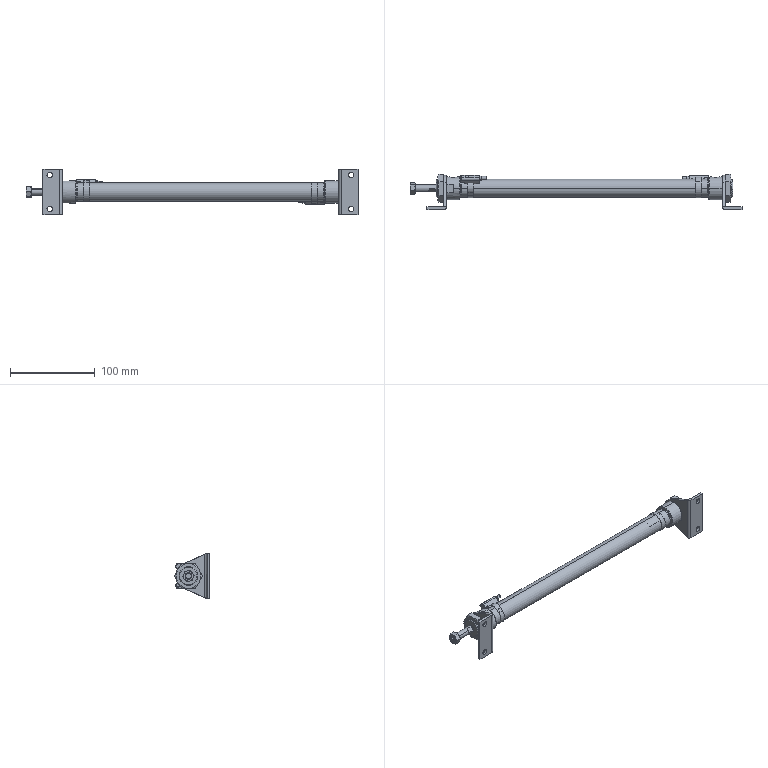Part | SolidWorks | 9 solids | 330 faces | box 392 x 41.5 x 54 mm | volume 88963 mm3 | plane 147 | cylinder 116 | cone 53 | spline 14 | commonest cylinder face diameters 3.4 x12 33 x12 2 x8 6.5 x8 16.4 x8 21.4 x6